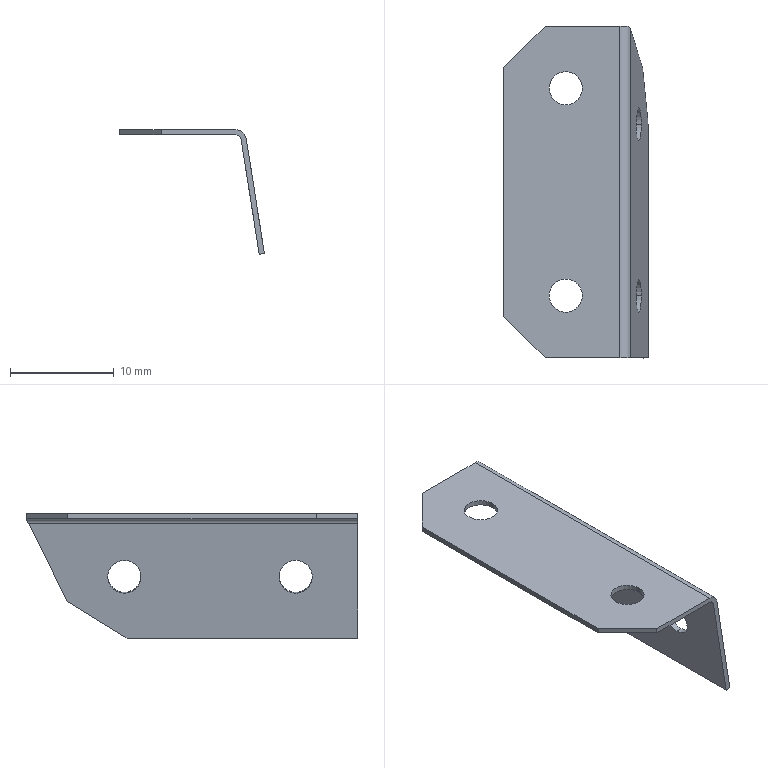Part | SolidWorks | features BaseBody 1 | 1 solid | 23 faces | box 13.963 x 32 x 12.004 mm | volume 331.486 mm3 | plane 12 | cylinder 10 | spline 1 | commonest cylinder face diameters 3.2 x8 1 x1 2 x1
STEP:
#1=CARTESIAN_POINT('',(-7.35,-10.,0.5));
#2=VERTEX_POINT('',#1);
#3=CARTESIAN_POINT('',(-4.15,-10.,0.5));
#4=VERTEX_POINT('',#3);
#5=CARTESIAN_POINT('',(-5.75,-10.,0.5));
#6=DIRECTION('',(0.,0.,1.));
#7=DIRECTION('',(-1.,0.,0.));
#8=AXIS2_PLACEMENT_3D('',#5,#6,#7);
#9=CIRCLE('',#8,1.6);
#10=EDGE_CURVE('',#2,#4,#9,.T.);
#11=ORIENTED_EDGE('',*,*,#10,.T.);
#12=CARTESIAN_POINT('',(-4.15,-10.,0.));
#13=VERTEX_POINT('',#12);
#14=CARTESIAN_POINT('',(-4.15,-10.,0.5));
#15=DIRECTION('',(0.,0.,-1.));
#16=VECTOR('',#15,1000.);
#17=LINE('',#14,#16);
#18=EDGE_CURVE('',#4,#13,#17,.T.);
#19=ORIENTED_EDGE('',*,*,#18,.T.);
#20=CARTESIAN_POINT('',(-7.35,-10.,0.));
#21=VERTEX_POINT('',#20);
#22=CARTESIAN_POINT('',(-5.75,-10.,0.));
#23=DIRECTION('',(0.,0.,-1.));
#24=DIRECTION('',(-1.,0.,0.));
#25=AXIS2_PLACEMENT_3D('',#22,#23,#24);
#26=CIRCLE('',#25,1.6);
#27=EDGE_CURVE('',#13,#21,#26,.T.);
#28=ORIENTED_EDGE('',*,*,#27,.T.);
#29=CARTESIAN_POINT('',(-7.35,-10.,0.5));
#30=DIRECTION('',(0.,0.,-1.));
#31=VECTOR('',#30,1000.);
#32=LINE('',#29,#31);
#33=EDGE_CURVE('',#2,#21,#32,.T.);
#34=ORIENTED_EDGE('',*,*,#33,.F.);
#35=EDGE_LOOP('',(#11,#19,#28,#34));
#36=FACE_OUTER_BOUND('',#35,.T.);
#37=CARTESIAN_POINT('',(-5.75,-10.,0.5));
#38=DIRECTION('',(0.,0.,-1.));
#39=DIRECTION('',(-1.,0.,0.));
#40=AXIS2_PLACEMENT_3D('',#37,#38,#39);
#41=CYLINDRICAL_SURFACE('',#40,1.6);
#42=ADVANCED_FACE('',(#36),#41,.F.);
#43=CARTESIAN_POINT('',(-7.35,10.,0.5));
#44=VERTEX_POINT('',#43);
#45=CARTESIAN_POINT('',(-4.15,10.,0.5));
#46=VERTEX_POINT('',#45);
#47=CARTESIAN_POINT('',(-5.75,10.,0.5));
#48=DIRECTION('',(0.,0.,1.));
#49=DIRECTION('',(-1.,0.,0.));
#50=AXIS2_PLACEMENT_3D('',#47,#48,#49);
#51=CIRCLE('',#50,1.6);
#52=EDGE_CURVE('',#44,#46,#51,.T.);
#53=ORIENTED_EDGE('',*,*,#52,.T.);
#54=CARTESIAN_POINT('',(-4.15,10.,0.));
#55=VERTEX_POINT('',#54);
#56=CARTESIAN_POINT('',(-4.15,10.,0.5));
#57=DIRECTION('',(0.,0.,-1.));
#58=VECTOR('',#57,1000.);
#59=LINE('',#56,#58);
#60=EDGE_CURVE('',#46,#55,#59,.T.);
#61=ORIENTED_EDGE('',*,*,#60,.T.);
#62=CARTESIAN_POINT('',(-7.35,10.,0.));
#63=VERTEX_POINT('',#62);
#64=CARTESIAN_POINT('',(-5.75,10.,0.));
#65=DIRECTION('',(0.,0.,1.));
#66=DIRECTION('',(-1.,0.,0.));
#67=AXIS2_PLACEMENT_3D('',#64,#65,#66);
#68=CIRCLE('',#67,1.6);
#69=EDGE_CURVE('',#63,#55,#68,.T.);
#70=ORIENTED_EDGE('',*,*,#69,.F.);
#71=CARTESIAN_POINT('',(-7.35,10.,0.5));
#72=DIRECTION('',(0.,0.,-1.));
#73=VECTOR('',#72,1000.);
#74=LINE('',#71,#73);
#75=EDGE_CURVE('',#44,#63,#74,.T.);
#76=ORIENTED_EDGE('',*,*,#75,.F.);
#77=EDGE_LOOP('',(#53,#61,#70,#76));
#78=FACE_OUTER_BOUND('',#77,.T.);
#79=CARTESIAN_POINT('',(-5.75,10.,0.5));
#80=DIRECTION('',(0.,0.,-1.));
#81=DIRECTION('',(-1.,0.,0.));
#82=AXIS2_PLACEMENT_3D('',#79,#80,#81);
#83=CYLINDRICAL_SURFACE('',#82,1.6);
#84=ADVANCED_FACE('',(#78),#83,.F.);
#85=CARTESIAN_POINT('',(1.024,-10.,-3.919));
#86=VERTEX_POINT('',#85);
#87=CARTESIAN_POINT('',(1.524,-10.,-7.079));
#88=VERTEX_POINT('',#87);
#89=CARTESIAN_POINT('',(1.274,-10.,-5.499));
#90=DIRECTION('',(0.9877,0.,0.1564));
#91=DIRECTION('',(-0.1564,0.,0.9877));
#92=AXIS2_PLACEMENT_3D('',#89,#90,#91);
#93=CIRCLE('',#92,1.6);
#94=EDGE_CURVE('',#86,#88,#93,.T.);
#95=ORIENTED_EDGE('',*,*,#94,.T.);
#96=CARTESIAN_POINT('',(1.031,-10.,-7.158));
#97=VERTEX_POINT('',#96);
#98=CARTESIAN_POINT('',(1.524,-10.,-7.079));
#99=DIRECTION('',(-0.9877,0.,-0.1564));
#100=VECTOR('',#99,1000.);
#101=LINE('',#98,#100);
#102=EDGE_CURVE('',#88,#97,#101,.T.);
#103=ORIENTED_EDGE('',*,*,#102,.T.);
#104=CARTESIAN_POINT('',(0.53,-10.,-3.997));
#105=VERTEX_POINT('',#104);
#106=CARTESIAN_POINT('',(0.7803,-10.,-5.577));
#107=DIRECTION('',(0.9877,0.,0.1564));
#108=DIRECTION('',(-0.1564,0.,0.9877));
#109=AXIS2_PLACEMENT_3D('',#106,#107,#108);
#110=CIRCLE('',#109,1.6);
#111=EDGE_CURVE('',#105,#97,#110,.T.);
#112=ORIENTED_EDGE('',*,*,#111,.F.);
#113=CARTESIAN_POINT('',(1.024,-10.,-3.919));
#114=DIRECTION('',(-0.9877,0.,-0.1564));
#115=VECTOR('',#114,1000.);
#116=LINE('',#113,#115);
#117=EDGE_CURVE('',#86,#105,#116,.T.);
#118=ORIENTED_EDGE('',*,*,#117,.F.);
#119=EDGE_LOOP('',(#95,#103,#112,#118));
#120=FACE_OUTER_BOUND('',#119,.T.);
#121=CARTESIAN_POINT('',(1.274,-10.,-5.499));
#122=DIRECTION('',(-0.9877,0.,-0.1564));
#123=DIRECTION('',(-0.1564,0.,0.9877));
#124=AXIS2_PLACEMENT_3D('',#121,#122,#123);
#125=CYLINDRICAL_SURFACE('',#124,1.6);
#126=ADVANCED_FACE('',(#120),#125,.F.);
#127=CARTESIAN_POINT('',(1.024,6.52,-3.919));
#128=VERTEX_POINT('',#127);
#129=CARTESIAN_POINT('',(1.524,6.52,-7.079));
#130=VERTEX_POINT('',#129);
#131=CARTESIAN_POINT('',(1.274,6.52,-5.499));
#132=DIRECTION('',(0.9877,0.,0.1564));
#133=DIRECTION('',(-0.1564,0.,0.9877));
#134=AXIS2_PLACEMENT_3D('',#131,#132,#133);
#135=CIRCLE('',#134,1.6);
#136=EDGE_CURVE('',#128,#130,#135,.T.);
#137=ORIENTED_EDGE('',*,*,#136,.T.);
#138=CARTESIAN_POINT('',(1.031,6.52,-7.158));
#139=VERTEX_POINT('',#138);
#140=CARTESIAN_POINT('',(1.524,6.52,-7.079));
#141=DIRECTION('',(-0.9877,0.,-0.1564));
#142=VECTOR('',#141,1000.);
#143=LINE('',#140,#142);
#144=EDGE_CURVE('',#130,#139,#143,.T.);
#145=ORIENTED_EDGE('',*,*,#144,.T.);
#146=CARTESIAN_POINT('',(0.53,6.52,-3.997));
#147=VERTEX_POINT('',#146);
#148=CARTESIAN_POINT('',(0.7803,6.52,-5.577));
#149=DIRECTION('',(0.9877,0.,0.1564));
#150=DIRECTION('',(-0.1564,0.,0.9877));
#151=AXIS2_PLACEMENT_3D('',#148,#149,#150);
#152=CIRCLE('',#151,1.6);
#153=EDGE_CURVE('',#147,#139,#152,.T.);
#154=ORIENTED_EDGE('',*,*,#153,.F.);
#155=CARTESIAN_POINT('',(1.024,6.52,-3.919));
#156=DIRECTION('',(-0.9877,0.,-0.1564));
#157=VECTOR('',#156,1000.);
#158=LINE('',#155,#157);
#159=EDGE_CURVE('',#128,#147,#158,.T.);
#160=ORIENTED_EDGE('',*,*,#159,.F.);
#161=EDGE_LOOP('',(#137,#145,#154,#160));
#162=FACE_OUTER_BOUND('',#161,.T.);
#163=CARTESIAN_POINT('',(1.274,6.52,-5.499));
#164=DIRECTION('',(-0.9877,0.,-0.1564));
#165=DIRECTION('',(-0.1564,0.,0.9877));
#166=AXIS2_PLACEMENT_3D('',#163,#164,#165);
#167=CYLINDRICAL_SURFACE('',#166,1.6);
#168=ADVANCED_FACE('',(#162),#167,.F.);
#169=ORIENTED_EDGE('',*,*,#18,.F.);
#170=CARTESIAN_POINT('',(-5.75,-10.,0.5));
#171=DIRECTION('',(0.,0.,1.));
#172=DIRECTION('',(-1.,0.,0.));
#173=AXIS2_PLACEMENT_3D('',#170,#171,#172);
#174=CIRCLE('',#173,1.6);
#175=EDGE_CURVE('',#4,#2,#174,.T.);
#176=ORIENTED_EDGE('',*,*,#175,.T.);
#177=ORIENTED_EDGE('',*,*,#33,.T.);
#178=CARTESIAN_POINT('',(-5.75,-10.,0.));
#179=DIRECTION('',(0.,0.,-1.));
#180=DIRECTION('',(-1.,0.,0.));
#181=AXIS2_PLACEMENT_3D('',#178,#179,#180);
#182=CIRCLE('',#181,1.6);
#183=EDGE_CURVE('',#21,#13,#182,.T.);
#184=ORIENTED_EDGE('',*,*,#183,.T.);
#185=EDGE_LOOP('',(#169,#176,#177,#184));
#186=FACE_OUTER_BOUND('',#185,.T.);
#187=CARTESIAN_POINT('',(-5.75,-10.,0.5));
#188=DIRECTION('',(0.,0.,-1.));
#189=DIRECTION('',(-1.,0.,0.));
#190=AXIS2_PLACEMENT_3D('',#187,#188,#189);
#191=CYLINDRICAL_SURFACE('',#190,1.6);
#192=ADVANCED_FACE('',(#186),#191,.F.);
#193=ORIENTED_EDGE('',*,*,#69,.T.);
#194=CARTESIAN_POINT('',(-5.75,10.,0.));
#195=DIRECTION('',(0.,0.,1.));
#196=DIRECTION('',(-1.,0.,0.));
#197=AXIS2_PLACEMENT_3D('',#194,#195,#196);
#198=CIRCLE('',#197,1.6);
#199=EDGE_CURVE('',#55,#63,#198,.T.);
#200=ORIENTED_EDGE('',*,*,#199,.T.);
#201=EDGE_LOOP('',(#193,#200));
#202=FACE_BOUND('',#201,.T.);
#203=ORIENTED_EDGE('',*,*,#183,.F.);
#204=ORIENTED_EDGE('',*,*,#27,.F.);
#205=EDGE_LOOP('',(#203,#204));
#206=FACE_BOUND('',#205,.T.);
#207=CARTESIAN_POINT('',(-7.75,16.,0.));
#208=VERTEX_POINT('',#207);
#209=CARTESIAN_POINT('',(-0.5301,16.,0.));
#210=VERTEX_POINT('',#209);
#211=CARTESIAN_POINT('',(-6.14,16.,0.));
#212=DIRECTION('',(1.,0.,0.));
#213=VECTOR('',#212,1000.);
#214=LINE('',#211,#213);
#215=EDGE_CURVE('',#208,#210,#214,.T.);
#216=ORIENTED_EDGE('',*,*,#215,.T.);
#217=CARTESIAN_POINT('',(-0.5301,-16.,0.));
#218=VERTEX_POINT('',#217);
#219=CARTESIAN_POINT('',(-0.5301,0.,0.));
#220=DIRECTION('',(0.,-1.,0.));
#221=VECTOR('',#220,1000.);
#222=LINE('',#219,#221);
#223=EDGE_CURVE('',#210,#218,#222,.T.);
#224=ORIENTED_EDGE('',*,*,#223,.T.);
#225=CARTESIAN_POINT('',(-7.75,-16.,0.));
#226=VERTEX_POINT('',#225);
#227=CARTESIAN_POINT('',(-6.14,-16.,0.));
#228=DIRECTION('',(-1.,0.,0.));
#229=VECTOR('',#228,1000.);
#230=LINE('',#227,#229);
#231=EDGE_CURVE('',#218,#226,#230,.T.);
#232=ORIENTED_EDGE('',*,*,#231,.T.);
#233=CARTESIAN_POINT('',(-11.75,-12.,0.));
#234=VERTEX_POINT('',#233);
#235=CARTESIAN_POINT('',(-7.75,-16.,0.));
#236=DIRECTION('',(-0.7071,0.7071,0.));
#237=VECTOR('',#236,1000.);
#238=LINE('',#235,#237);
#239=EDGE_CURVE('',#226,#234,#238,.T.);
#240=ORIENTED_EDGE('',*,*,#239,.T.);
#241=CARTESIAN_POINT('',(-11.75,12.,0.));
#242=VERTEX_POINT('',#241);
#243=CARTESIAN_POINT('',(-11.75,0.,0.));
#244=DIRECTION('',(0.,1.,0.));
#245=VECTOR('',#244,1000.);
#246=LINE('',#243,#245);
#247=EDGE_CURVE('',#234,#242,#246,.T.);
#248=ORIENTED_EDGE('',*,*,#247,.T.);
#249=CARTESIAN_POINT('',(-11.75,12.,0.));
#250=DIRECTION('',(0.7071,0.7071,0.));
#251=VECTOR('',#250,1000.);
#252=LINE('',#249,#251);
#253=EDGE_CURVE('',#242,#208,#252,.T.);
#254=ORIENTED_EDGE('',*,*,#253,.T.);
#255=EDGE_LOOP('',(#216,#224,#232,#240,#248,#254));
#256=FACE_OUTER_BOUND('',#255,.T.);
#257=CARTESIAN_POINT('',(-11.75,16.,0.));
#258=DIRECTION('',(0.,0.,-1.));
#259=DIRECTION('',(1.,0.,0.));
#260=AXIS2_PLACEMENT_3D('',#257,#258,#259);
#261=PLANE('',#260);
#262=ADVANCED_FACE('',(#202,#206,#256),#261,.T.);
#263=ORIENTED_EDGE('',*,*,#52,.F.);
#264=CARTESIAN_POINT('',(-5.75,10.,0.5));
#265=DIRECTION('',(0.,0.,1.));
#266=DIRECTION('',(-1.,0.,0.));
#267=AXIS2_PLACEMENT_3D('',#264,#265,#266);
#268=CIRCLE('',#267,1.6);
#269=EDGE_CURVE('',#46,#44,#268,.T.);
#270=ORIENTED_EDGE('',*,*,#269,.F.);
#271=EDGE_LOOP('',(#263,#270));
#272=FACE_BOUND('',#271,.T.);
#273=ORIENTED_EDGE('',*,*,#10,.F.);
#274=ORIENTED_EDGE('',*,*,#175,.F.);
#275=EDGE_LOOP('',(#273,#274));
#276=FACE_BOUND('',#275,.T.);
#277=CARTESIAN_POINT('',(-7.75,16.,0.5));
#278=VERTEX_POINT('',#277);
#279=CARTESIAN_POINT('',(-0.5301,16.,0.5));
#280=VERTEX_POINT('',#279);
#281=CARTESIAN_POINT('',(-6.14,16.,0.5));
#282=DIRECTION('',(1.,0.,0.));
#283=VECTOR('',#282,1000.);
#284=LINE('',#281,#283);
#285=EDGE_CURVE('',#278,#280,#284,.T.);
#286=ORIENTED_EDGE('',*,*,#285,.F.);
#287=CARTESIAN_POINT('',(-11.75,12.,0.5));
#288=VERTEX_POINT('',#287);
#289=CARTESIAN_POINT('',(-7.75,16.,0.5));
#290=DIRECTION('',(0.7071,0.7071,0.));
#291=VECTOR('',#290,1000.);
#292=LINE('',#289,#291);
#293=EDGE_CURVE('',#288,#278,#292,.T.);
#294=ORIENTED_EDGE('',*,*,#293,.F.);
#295=CARTESIAN_POINT('',(-11.75,-12.,0.5));
#296=VERTEX_POINT('',#295);
#297=CARTESIAN_POINT('',(-11.75,0.,0.5));
#298=DIRECTION('',(0.,1.,0.));
#299=VECTOR('',#298,1000.);
#300=LINE('',#297,#299);
#301=EDGE_CURVE('',#296,#288,#300,.T.);
#302=ORIENTED_EDGE('',*,*,#301,.F.);
#303=CARTESIAN_POINT('',(-7.75,-16.,0.5));
#304=VERTEX_POINT('',#303);
#305=CARTESIAN_POINT('',(-11.75,-12.,0.5));
#306=DIRECTION('',(-0.7071,0.7071,0.));
#307=VECTOR('',#306,1000.);
#308=LINE('',#305,#307);
#309=EDGE_CURVE('',#304,#296,#308,.T.);
#310=ORIENTED_EDGE('',*,*,#309,.F.);
#311=CARTESIAN_POINT('',(-0.5301,-16.,0.5));
#312=VERTEX_POINT('',#311);
#313=CARTESIAN_POINT('',(-6.14,-16.,0.5));
#314=DIRECTION('',(-1.,0.,0.));
#315=VECTOR('',#314,1000.);
#316=LINE('',#313,#315);
#317=EDGE_CURVE('',#312,#304,#316,.T.);
#318=ORIENTED_EDGE('',*,*,#317,.F.);
#319=CARTESIAN_POINT('',(-0.5301,0.,0.5));
#320=DIRECTION('',(0.,-1.,0.));
#321=VECTOR('',#320,1000.);
#322=LINE('',#319,#321);
#323=EDGE_CURVE('',#280,#312,#322,.T.);
#324=ORIENTED_EDGE('',*,*,#323,.F.);
#325=EDGE_LOOP('',(#286,#294,#302,#310,#318,#324));
#326=FACE_OUTER_BOUND('',#325,.T.);
#327=CARTESIAN_POINT('',(-11.75,16.,0.5));
#328=DIRECTION('',(0.,0.,-1.));
#329=DIRECTION('',(1.,0.,0.));
#330=AXIS2_PLACEMENT_3D('',#327,#328,#329);
#331=PLANE('',#330);
#332=ADVANCED_FACE('',(#272,#276,#326),#331,.F.);
#333=ORIENTED_EDGE('',*,*,#60,.F.);
#334=ORIENTED_EDGE('',*,*,#269,.T.);
#335=ORIENTED_EDGE('',*,*,#75,.T.);
#336=ORIENTED_EDGE('',*,*,#199,.F.);
#337=EDGE_LOOP('',(#333,#334,#335,#336));
#338=FACE_OUTER_BOUND('',#337,.T.);
#339=CARTESIAN_POINT('',(-5.75,10.,0.5));
#340=DIRECTION('',(0.,0.,-1.));
#341=DIRECTION('',(-1.,0.,0.));
#342=AXIS2_PLACEMENT_3D('',#339,#340,#341);
#343=CYLINDRICAL_SURFACE('',#342,1.6);
#344=ADVANCED_FACE('',(#338),#343,.F.);
#345=ORIENTED_EDGE('',*,*,#223,.F.);
#346=CARTESIAN_POINT('',(-0.2054,16.,-0.1198));
#347=VERTEX_POINT('',#346);
#348=CARTESIAN_POINT('',(-0.5301,16.,-0.5));
#349=DIRECTION('',(0.,1.,0.));
#350=DIRECTION('',(0.,0.,-1.));
#351=AXIS2_PLACEMENT_3D('',#348,#349,#350);
#352=CIRCLE('',#351,0.5);
#353=EDGE_CURVE('',#210,#347,#352,.T.);
#354=ORIENTED_EDGE('',*,*,#353,.T.);
#355=CARTESIAN_POINT('',(-0.0363,15.741,-0.4218));
#356=VERTEX_POINT('',#355);
#357=CARTESIAN_POINT('',(-0.2054,16.,-0.1198));
#358=CARTESIAN_POINT('',(-0.1155,15.914,-0.1966));
#359=CARTESIAN_POINT('',(-0.05479,15.828,-0.305));
#360=CARTESIAN_POINT('',(-0.0363,15.741,-0.4218));
#361=B_SPLINE_CURVE_WITH_KNOTS('',3,(#357,#358,#359,#360),.UNSPECIFIED.,.F.,.F.,(4,4),(0.,0.0004379),.UNSPECIFIED.);
#362=EDGE_CURVE('',#347,#356,#361,.T.);
#363=ORIENTED_EDGE('',*,*,#362,.T.);
#364=CARTESIAN_POINT('',(-0.0363,-16.,-0.4218));
#365=VERTEX_POINT('',#364);
#366=CARTESIAN_POINT('',(-0.0363,0.,-0.4218));
#367=DIRECTION('',(0.,-1.,0.));
#368=VECTOR('',#367,1000.);
#369=LINE('',#366,#368);
#370=EDGE_CURVE('',#356,#365,#369,.T.);
#371=ORIENTED_EDGE('',*,*,#370,.T.);
#372=CARTESIAN_POINT('',(-0.5301,-16.,-0.5));
#373=DIRECTION('',(0.,-1.,0.));
#374=DIRECTION('',(0.,0.,-1.));
#375=AXIS2_PLACEMENT_3D('',#372,#373,#374);
#376=CIRCLE('',#375,0.5);
#377=EDGE_CURVE('',#365,#218,#376,.T.);
#378=ORIENTED_EDGE('',*,*,#377,.T.);
#379=EDGE_LOOP('',(#345,#354,#363,#371,#378));
#380=FACE_OUTER_BOUND('',#379,.T.);
#381=CARTESIAN_POINT('',(-0.5301,16.,-0.5));
#382=DIRECTION('',(0.,-1.,0.));
#383=DIRECTION('',(0.,0.,-1.));
#384=AXIS2_PLACEMENT_3D('',#381,#382,#383);
#385=CYLINDRICAL_SURFACE('',#384,0.5);
#386=ADVANCED_FACE('',(#380),#385,.F.);
#387=ORIENTED_EDGE('',*,*,#285,.T.);
#388=CARTESIAN_POINT('',(0.1193,16.,0.2604));
#389=VERTEX_POINT('',#388);
#390=CARTESIAN_POINT('',(-0.5301,16.,-0.5));
#391=DIRECTION('',(0.,1.,0.));
#392=DIRECTION('',(0.,0.,-1.));
#393=AXIS2_PLACEMENT_3D('',#390,#391,#392);
#394=CIRCLE('',#393,1.);
#395=EDGE_CURVE('',#280,#389,#394,.T.);
#396=ORIENTED_EDGE('',*,*,#395,.T.);
#397=CARTESIAN_POINT('',(0.1193,16.,0.2604));
#398=DIRECTION('',(-0.6494,0.,-0.7604));
#399=VECTOR('',#398,1000.);
#400=LINE('',#397,#399);
#401=EDGE_CURVE('',#389,#347,#400,.T.);
#402=ORIENTED_EDGE('',*,*,#401,.T.);
#403=ORIENTED_EDGE('',*,*,#353,.F.);
#404=ORIENTED_EDGE('',*,*,#215,.F.);
#405=CARTESIAN_POINT('',(-7.75,16.,0.25));
#406=DIRECTION('',(0.,0.,1.));
#407=VECTOR('',#406,1000.);
#408=LINE('',#405,#407);
#409=EDGE_CURVE('',#208,#278,#408,.T.);
#410=ORIENTED_EDGE('',*,*,#409,.T.);
#411=EDGE_LOOP('',(#387,#396,#402,#403,#404,#410));
#412=FACE_OUTER_BOUND('',#411,.T.);
#413=CARTESIAN_POINT('',(-0.5301,16.,0.5));
#414=DIRECTION('',(0.,1.,0.));
#415=DIRECTION('',(0.,0.,-1.));
#416=AXIS2_PLACEMENT_3D('',#413,#414,#415);
#417=PLANE('',#416);
#418=ADVANCED_FACE('',(#412),#417,.T.);
#419=ORIENTED_EDGE('',*,*,#293,.T.);
#420=ORIENTED_EDGE('',*,*,#409,.F.);
#421=ORIENTED_EDGE('',*,*,#253,.F.);
#422=CARTESIAN_POINT('',(-11.75,12.,0.25));
#423=DIRECTION('',(0.,0.,1.));
#424=VECTOR('',#423,1000.);
#425=LINE('',#422,#424);
#426=EDGE_CURVE('',#242,#288,#425,.T.);
#427=ORIENTED_EDGE('',*,*,#426,.T.);
#428=EDGE_LOOP('',(#419,#420,#421,#427));
#429=FACE_OUTER_BOUND('',#428,.T.);
#430=CARTESIAN_POINT('',(-7.75,16.,0.));
#431=DIRECTION('',(-0.7071,0.7071,0.));
#432=DIRECTION('',(-0.7071,-0.7071,0.));
#433=AXIS2_PLACEMENT_3D('',#430,#431,#432);
#434=PLANE('',#433);
#435=ADVANCED_FACE('',(#429),#434,.T.);
#436=ORIENTED_EDGE('',*,*,#301,.T.);
#437=ORIENTED_EDGE('',*,*,#426,.F.);
#438=ORIENTED_EDGE('',*,*,#247,.F.);
#439=CARTESIAN_POINT('',(-11.75,-12.,0.25));
#440=DIRECTION('',(0.,0.,1.));
#441=VECTOR('',#440,1000.);
#442=LINE('',#439,#441);
#443=EDGE_CURVE('',#234,#296,#442,.T.);
#444=ORIENTED_EDGE('',*,*,#443,.T.);
#445=EDGE_LOOP('',(#436,#437,#438,#444));
#446=FACE_OUTER_BOUND('',#445,.T.);
#447=CARTESIAN_POINT('',(-11.75,12.,0.));
#448=DIRECTION('',(-1.,0.,0.));
#449=DIRECTION('',(0.,-1.,0.));
#450=AXIS2_PLACEMENT_3D('',#447,#448,#449);
#451=PLANE('',#450);
#452=ADVANCED_FACE('',(#446),#451,.T.);
#453=ORIENTED_EDGE('',*,*,#309,.T.);
#454=ORIENTED_EDGE('',*,*,#443,.F.);
#455=ORIENTED_EDGE('',*,*,#239,.F.);
#456=CARTESIAN_POINT('',(-7.75,-16.,0.25));
#457=DIRECTION('',(0.,0.,1.));
#458=VECTOR('',#457,1000.);
#459=LINE('',#456,#458);
#460=EDGE_CURVE('',#226,#304,#459,.T.);
#461=ORIENTED_EDGE('',*,*,#460,.T.);
#462=EDGE_LOOP('',(#453,#454,#455,#461));
#463=FACE_OUTER_BOUND('',#462,.T.);
#464=CARTESIAN_POINT('',(-11.75,-12.,0.));
#465=DIRECTION('',(-0.7071,-0.7071,0.));
#466=DIRECTION('',(0.7071,-0.7071,0.));
#467=AXIS2_PLACEMENT_3D('',#464,#465,#466);
#468=PLANE('',#467);
#469=ADVANCED_FACE('',(#463),#468,.T.);
#470=ORIENTED_EDGE('',*,*,#231,.F.);
#471=ORIENTED_EDGE('',*,*,#377,.F.);
#472=CARTESIAN_POINT('',(1.719,-16.,-11.504));
#473=VERTEX_POINT('',#472);
#474=CARTESIAN_POINT('',(0.8413,-16.,-5.963));
#475=DIRECTION('',(-0.1564,0.,0.9877));
#476=VECTOR('',#475,1000.);
#477=LINE('',#474,#476);
#478=EDGE_CURVE('',#473,#365,#477,.T.);
#479=ORIENTED_EDGE('',*,*,#478,.F.);
#480=CARTESIAN_POINT('',(2.213,-16.,-11.425));
#481=VERTEX_POINT('',#480);
#482=CARTESIAN_POINT('',(1.966,-16.,-11.464));
#483=DIRECTION('',(0.9877,0.,0.1564));
#484=VECTOR('',#483,1000.);
#485=LINE('',#482,#484);
#486=EDGE_CURVE('',#473,#481,#485,.T.);
#487=ORIENTED_EDGE('',*,*,#486,.T.);
#488=CARTESIAN_POINT('',(0.4575,-16.,-0.3436));
#489=VERTEX_POINT('',#488);
#490=CARTESIAN_POINT('',(1.335,-16.,-5.884));
#491=DIRECTION('',(-0.1564,0.,0.9877));
#492=VECTOR('',#491,1000.);
#493=LINE('',#490,#492);
#494=EDGE_CURVE('',#481,#489,#493,.T.);
#495=ORIENTED_EDGE('',*,*,#494,.T.);
#496=CARTESIAN_POINT('',(-0.5301,-16.,-0.5));
#497=DIRECTION('',(0.,-1.,0.));
#498=DIRECTION('',(0.,0.,-1.));
#499=AXIS2_PLACEMENT_3D('',#496,#497,#498);
#500=CIRCLE('',#499,1.);
#501=EDGE_CURVE('',#489,#312,#500,.T.);
#502=ORIENTED_EDGE('',*,*,#501,.T.);
#503=ORIENTED_EDGE('',*,*,#317,.T.);
#504=ORIENTED_EDGE('',*,*,#460,.F.);
#505=EDGE_LOOP('',(#470,#471,#479,#487,#495,#502,#503,#504));
#506=FACE_OUTER_BOUND('',#505,.T.);
#507=CARTESIAN_POINT('',(-7.75,-16.,0.));
#508=DIRECTION('',(0.,-1.,0.));
#509=DIRECTION('',(1.,0.,0.));
#510=AXIS2_PLACEMENT_3D('',#507,#508,#509);
#511=PLANE('',#510);
#512=ADVANCED_FACE('',(#506),#511,.T.);
#513=ORIENTED_EDGE('',*,*,#395,.F.);
#514=ORIENTED_EDGE('',*,*,#323,.T.);
#515=ORIENTED_EDGE('',*,*,#501,.F.);
#516=CARTESIAN_POINT('',(0.4575,15.741,-0.3436));
#517=VERTEX_POINT('',#516);
#518=CARTESIAN_POINT('',(0.4575,0.,-0.3436));
#519=DIRECTION('',(0.,-1.,0.));
#520=VECTOR('',#519,1000.);
#521=LINE('',#518,#520);
#522=EDGE_CURVE('',#517,#489,#521,.T.);
#523=ORIENTED_EDGE('',*,*,#522,.F.);
#524=CARTESIAN_POINT('',(0.1193,16.,0.2604));
#525=CARTESIAN_POINT('',(0.2094,15.957,0.1835));
#526=CARTESIAN_POINT('',(0.2852,15.914,0.091));
#527=CARTESIAN_POINT('',(0.4007,15.827,-0.1159));
#528=CARTESIAN_POINT('',(0.439,15.785,-0.2265));
#529=CARTESIAN_POINT('',(0.4575,15.741,-0.3436));
#530=B_SPLINE_CURVE_WITH_KNOTS('',3,(#524,#525,#526,#527,#528,#529),.UNSPECIFIED.,.F.,.F.,(4,2,4),(0.,0.0003772,0.0007544),.UNSPECIFIED.);
#531=EDGE_CURVE('',#389,#517,#530,.T.);
#532=ORIENTED_EDGE('',*,*,#531,.F.);
#533=EDGE_LOOP('',(#513,#514,#515,#523,#532));
#534=FACE_OUTER_BOUND('',#533,.T.);
#535=CARTESIAN_POINT('',(-0.5301,16.,-0.5));
#536=DIRECTION('',(0.,-1.,0.));
#537=DIRECTION('',(0.,0.,-1.));
#538=AXIS2_PLACEMENT_3D('',#535,#536,#537);
#539=CYLINDRICAL_SURFACE('',#538,1.);
#540=ADVANCED_FACE('',(#534),#539,.T.);
#541=ORIENTED_EDGE('',*,*,#111,.T.);
#542=CARTESIAN_POINT('',(0.7803,-10.,-5.577));
#543=DIRECTION('',(0.9877,0.,0.1564));
#544=DIRECTION('',(-0.1564,0.,0.9877));
#545=AXIS2_PLACEMENT_3D('',#542,#543,#544);
#546=CIRCLE('',#545,1.6);
#547=EDGE_CURVE('',#97,#105,#546,.T.);
#548=ORIENTED_EDGE('',*,*,#547,.T.);
#549=EDGE_LOOP('',(#541,#548));
#550=FACE_BOUND('',#549,.T.);
#551=ORIENTED_EDGE('',*,*,#153,.T.);
#552=CARTESIAN_POINT('',(0.7803,6.52,-5.577));
#553=DIRECTION('',(0.9877,0.,0.1564));
#554=DIRECTION('',(-0.1564,0.,0.9877));
#555=AXIS2_PLACEMENT_3D('',#552,#553,#554);
#556=CIRCLE('',#555,1.6);
#557=EDGE_CURVE('',#139,#147,#556,.T.);
#558=ORIENTED_EDGE('',*,*,#557,.T.);
#559=EDGE_LOOP('',(#551,#558));
#560=FACE_BOUND('',#559,.T.);
#561=CARTESIAN_POINT('',(1.719,6.269,-11.504));
#562=VERTEX_POINT('',#561);
#563=CARTESIAN_POINT('',(1.719,-0.03406,-11.504));
#564=DIRECTION('',(0.,-1.,0.));
#565=VECTOR('',#564,1000.);
#566=LINE('',#563,#565);
#567=EDGE_CURVE('',#562,#473,#566,.T.);
#568=ORIENTED_EDGE('',*,*,#567,.T.);
#569=ORIENTED_EDGE('',*,*,#478,.T.);
#570=ORIENTED_EDGE('',*,*,#370,.F.);
#571=CARTESIAN_POINT('',(1.156,12.023,-7.953));
#572=VERTEX_POINT('',#571);
#573=CARTESIAN_POINT('',(-0.0363,15.741,-0.4218));
#574=DIRECTION('',(0.1406,-0.4384,-0.8877));
#575=VECTOR('',#574,1000.);
#576=LINE('',#573,#575);
#577=EDGE_CURVE('',#356,#572,#576,.T.);
#578=ORIENTED_EDGE('',*,*,#577,.T.);
#579=CARTESIAN_POINT('',(1.156,12.023,-7.953));
#580=DIRECTION('',(0.0829,-0.848,-0.5234));
#581=VECTOR('',#580,1000.);
#582=LINE('',#579,#581);
#583=EDGE_CURVE('',#572,#562,#582,.T.);
#584=ORIENTED_EDGE('',*,*,#583,.T.);
#585=EDGE_LOOP('',(#568,#569,#570,#578,#584));
#586=FACE_OUTER_BOUND('',#585,.T.);
#587=CARTESIAN_POINT('',(-0.0363,15.932,-0.4218));
#588=DIRECTION('',(-0.9877,0.,-0.1564));
#589=DIRECTION('',(0.1564,0.,-0.9877));
#590=AXIS2_PLACEMENT_3D('',#587,#588,#589);
#591=PLANE('',#590);
#592=ADVANCED_FACE('',(#550,#560,#586),#591,.T.);
#593=ORIENTED_EDGE('',*,*,#531,.T.);
#594=CARTESIAN_POINT('',(0.2106,15.741,-0.3827));
#595=DIRECTION('',(0.9877,0.,0.1564));
#596=VECTOR('',#595,1000.);
#597=LINE('',#594,#596);
#598=EDGE_CURVE('',#356,#517,#597,.T.);
#599=ORIENTED_EDGE('',*,*,#598,.F.);
#600=ORIENTED_EDGE('',*,*,#362,.F.);
#601=ORIENTED_EDGE('',*,*,#401,.F.);
#602=EDGE_LOOP('',(#593,#599,#600,#601));
#603=FACE_OUTER_BOUND('',#602,.T.);
#604=CARTESIAN_POINT('',(0.1218,16.,0.2648));
#605=CARTESIAN_POINT('',(0.1221,16.,0.2646));
#606=CARTESIAN_POINT('',(0.1223,16.,0.2644));
#607=CARTESIAN_POINT('',(0.1226,16.,0.2642));
#608=CARTESIAN_POINT('',(0.3033,15.913,0.1098));
#609=CARTESIAN_POINT('',(0.4253,15.828,-0.108));
#610=CARTESIAN_POINT('',(0.4625,15.741,-0.3428));
#611=CARTESIAN_POINT('',(0.1186,16.,0.261));
#612=CARTESIAN_POINT('',(0.1188,16.,0.2608));
#613=CARTESIAN_POINT('',(0.1191,16.,0.2606));
#614=CARTESIAN_POINT('',(0.1193,16.,0.2604));
#615=CARTESIAN_POINT('',(0.2992,15.913,0.1068));
#616=CARTESIAN_POINT('',(0.4205,15.828,-0.1099));
#617=CARTESIAN_POINT('',(0.4575,15.741,-0.3436));
#618=CARTESIAN_POINT('',(-0.2058,16.,-0.1195));
#619=CARTESIAN_POINT('',(-0.2057,16.,-0.1196));
#620=CARTESIAN_POINT('',(-0.2055,16.,-0.1197));
#621=CARTESIAN_POINT('',(-0.2054,16.,-0.1198));
#622=CARTESIAN_POINT('',(-0.1155,15.914,-0.1966));
#623=CARTESIAN_POINT('',(-0.05479,15.828,-0.305));
#624=CARTESIAN_POINT('',(-0.0363,15.741,-0.4218));
#625=B_SPLINE_SURFACE_WITH_KNOTS('',1,3,((#604,#605,#606,#607,#608,#609,#610),(#611,#612,#613,#614,#615,#616,#617),(#618,#619,#620,#621,#622,#623,#624)),.UNSPECIFIED.,.F.,.F.,.F.,(2,1,2),(4,3,4),(-0.01,0.,1.),(-0.001366,0.,1.),.UNSPECIFIED.);
#626=ADVANCED_FACE('',(#603),#625,.F.);
#627=ORIENTED_EDGE('',*,*,#136,.F.);
#628=CARTESIAN_POINT('',(1.274,6.52,-5.499));
#629=DIRECTION('',(0.9877,0.,0.1564));
#630=DIRECTION('',(-0.1564,0.,0.9877));
#631=AXIS2_PLACEMENT_3D('',#628,#629,#630);
#632=CIRCLE('',#631,1.6);
#633=EDGE_CURVE('',#130,#128,#632,.T.);
#634=ORIENTED_EDGE('',*,*,#633,.F.);
#635=EDGE_LOOP('',(#627,#634));
#636=FACE_BOUND('',#635,.T.);
#637=ORIENTED_EDGE('',*,*,#94,.F.);
#638=CARTESIAN_POINT('',(1.274,-10.,-5.499));
#639=DIRECTION('',(0.9877,0.,0.1564));
#640=DIRECTION('',(-0.1564,0.,0.9877));
#641=AXIS2_PLACEMENT_3D('',#638,#639,#640);
#642=CIRCLE('',#641,1.6);
#643=EDGE_CURVE('',#88,#86,#642,.T.);
#644=ORIENTED_EDGE('',*,*,#643,.F.);
#645=EDGE_LOOP('',(#637,#644));
#646=FACE_BOUND('',#645,.T.);
#647=CARTESIAN_POINT('',(2.213,6.269,-11.425));
#648=VERTEX_POINT('',#647);
#649=CARTESIAN_POINT('',(2.213,-0.03406,-11.425));
#650=DIRECTION('',(0.,-1.,0.));
#651=VECTOR('',#650,1000.);
#652=LINE('',#649,#651);
#653=EDGE_CURVE('',#648,#481,#652,.T.);
#654=ORIENTED_EDGE('',*,*,#653,.F.);
#655=CARTESIAN_POINT('',(1.65,12.023,-7.874));
#656=VERTEX_POINT('',#655);
#657=CARTESIAN_POINT('',(2.213,6.269,-11.425));
#658=DIRECTION('',(0.0829,-0.848,-0.5234));
#659=VECTOR('',#658,1000.);
#660=LINE('',#657,#659);
#661=EDGE_CURVE('',#656,#648,#660,.T.);
#662=ORIENTED_EDGE('',*,*,#661,.F.);
#663=CARTESIAN_POINT('',(1.65,12.023,-7.874));
#664=DIRECTION('',(0.1406,-0.4384,-0.8877));
#665=VECTOR('',#664,1000.);
#666=LINE('',#663,#665);
#667=EDGE_CURVE('',#517,#656,#666,.T.);
#668=ORIENTED_EDGE('',*,*,#667,.F.);
#669=ORIENTED_EDGE('',*,*,#522,.T.);
#670=ORIENTED_EDGE('',*,*,#494,.F.);
#671=EDGE_LOOP('',(#654,#662,#668,#669,#670));
#672=FACE_OUTER_BOUND('',#671,.T.);
#673=CARTESIAN_POINT('',(0.4575,15.932,-0.3436));
#674=DIRECTION('',(-0.9877,0.,-0.1564));
#675=DIRECTION('',(0.1564,0.,-0.9877));
#676=AXIS2_PLACEMENT_3D('',#673,#674,#675);
#677=PLANE('',#676);
#678=ADVANCED_FACE('',(#636,#646,#672),#677,.F.);
#679=ORIENTED_EDGE('',*,*,#102,.F.);
#680=ORIENTED_EDGE('',*,*,#643,.T.);
#681=ORIENTED_EDGE('',*,*,#117,.T.);
#682=ORIENTED_EDGE('',*,*,#547,.F.);
#683=EDGE_LOOP('',(#679,#680,#681,#682));
#684=FACE_OUTER_BOUND('',#683,.T.);
#685=CARTESIAN_POINT('',(1.274,-10.,-5.499));
#686=DIRECTION('',(-0.9877,0.,-0.1564));
#687=DIRECTION('',(-0.1564,0.,0.9877));
#688=AXIS2_PLACEMENT_3D('',#685,#686,#687);
#689=CYLINDRICAL_SURFACE('',#688,1.6);
#690=ADVANCED_FACE('',(#684),#689,.F.);
#691=ORIENTED_EDGE('',*,*,#144,.F.);
#692=ORIENTED_EDGE('',*,*,#633,.T.);
#693=ORIENTED_EDGE('',*,*,#159,.T.);
#694=ORIENTED_EDGE('',*,*,#557,.F.);
#695=EDGE_LOOP('',(#691,#692,#693,#694));
#696=FACE_OUTER_BOUND('',#695,.T.);
#697=CARTESIAN_POINT('',(1.274,6.52,-5.499));
#698=DIRECTION('',(-0.9877,0.,-0.1564));
#699=DIRECTION('',(-0.1564,0.,0.9877));
#700=AXIS2_PLACEMENT_3D('',#697,#698,#699);
#701=CYLINDRICAL_SURFACE('',#700,1.6);
#702=ADVANCED_FACE('',(#696),#701,.F.);
#703=ORIENTED_EDGE('',*,*,#653,.T.);
#704=ORIENTED_EDGE('',*,*,#486,.F.);
#705=ORIENTED_EDGE('',*,*,#567,.F.);
#706=CARTESIAN_POINT('',(1.966,6.269,-11.464));
#707=DIRECTION('',(0.9877,0.,0.1564));
#708=VECTOR('',#707,1000.);
#709=LINE('',#706,#708);
#710=EDGE_CURVE('',#562,#648,#709,.T.);
#711=ORIENTED_EDGE('',*,*,#710,.T.);
#712=EDGE_LOOP('',(#703,#704,#705,#711));
#713=FACE_OUTER_BOUND('',#712,.T.);
#714=CARTESIAN_POINT('',(1.719,-16.,-11.504));
#715=DIRECTION('',(0.1564,0.,-0.9877));
#716=DIRECTION('',(0.,1.,0.));
#717=AXIS2_PLACEMENT_3D('',#714,#715,#716);
#718=PLANE('',#717);
#719=ADVANCED_FACE('',(#713),#718,.T.);
#720=ORIENTED_EDGE('',*,*,#661,.T.);
#721=ORIENTED_EDGE('',*,*,#710,.F.);
#722=ORIENTED_EDGE('',*,*,#583,.F.);
#723=CARTESIAN_POINT('',(1.403,12.023,-7.913));
#724=DIRECTION('',(0.9877,0.,0.1564));
#725=VECTOR('',#724,1000.);
#726=LINE('',#723,#725);
#727=EDGE_CURVE('',#572,#656,#726,.T.);
#728=ORIENTED_EDGE('',*,*,#727,.T.);
#729=EDGE_LOOP('',(#720,#721,#722,#728));
#730=FACE_OUTER_BOUND('',#729,.T.);
#731=CARTESIAN_POINT('',(1.719,6.269,-11.504));
#732=DIRECTION('',(0.1327,0.5299,-0.8376));
#733=DIRECTION('',(-0.0829,0.848,0.5234));
#734=AXIS2_PLACEMENT_3D('',#731,#732,#733);
#735=PLANE('',#734);
#736=ADVANCED_FACE('',(#730),#735,.T.);
#737=ORIENTED_EDGE('',*,*,#727,.F.);
#738=ORIENTED_EDGE('',*,*,#577,.F.);
#739=ORIENTED_EDGE('',*,*,#598,.T.);
#740=ORIENTED_EDGE('',*,*,#667,.T.);
#741=EDGE_LOOP('',(#737,#738,#739,#740));
#742=FACE_OUTER_BOUND('',#741,.T.);
#743=CARTESIAN_POINT('',(1.156,12.023,-7.953));
#744=DIRECTION('',(0.06858,0.8988,-0.433));
#745=DIRECTION('',(-0.1406,0.4384,0.8877));
#746=AXIS2_PLACEMENT_3D('',#743,#744,#745);
#747=PLANE('',#746);
#748=ADVANCED_FACE('',(#742),#747,.T.);
#749=CLOSED_SHELL('',(#42,#84,#126,#168,#192,#262,#332,#344,#386,#418,#435,#452,#469,#512,#540,#592,#626,#678,#690,#702,#719,#736,#748));
#750=MANIFOLD_SOLID_BREP('',#749);
#751=CARTESIAN_POINT('',(0.,0.,0.));
#752=DIRECTION('',(0.,0.,1.));
#753=DIRECTION('',(1.,0.,0.));
#754=AXIS2_PLACEMENT_3D('',#751,#752,#753);
#755=(LENGTH_UNIT()NAMED_UNIT(*)SI_UNIT(.MILLI.,.METRE.));
#756=UNCERTAINTY_MEASURE_WITH_UNIT(LENGTH_MEASURE(0.00001),#755,'','');
#757=(NAMED_UNIT(*)PLANE_ANGLE_UNIT()SI_UNIT($,.RADIAN.));
#758=(NAMED_UNIT(*)SI_UNIT($,.STERADIAN.)SOLID_ANGLE_UNIT());
#759=(GEOMETRIC_REPRESENTATION_CONTEXT(3)GLOBAL_UNCERTAINTY_ASSIGNED_CONTEXT((#756))GLOBAL_UNIT_ASSIGNED_CONTEXT((#755,#757,#758))REPRESENTATION_CONTEXT('',''));
#760=ADVANCED_BREP_SHAPE_REPRESENTATION('',(#750,#754),#759);